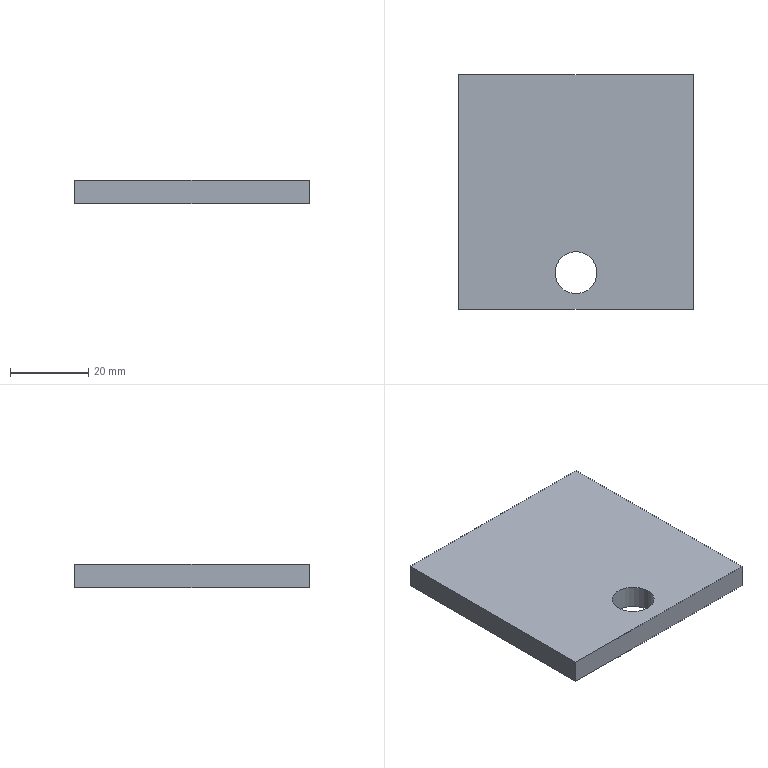Part | NX | features 凸台-拉伸21[3] 2 | 1 solid | 8 faces | box 60 x 60 x 6 mm | volume 21058 mm3 | plane 6 | cylinder 2 | commonest cylinder face diameters 10.72 x2
STEP:
#1=CARTESIAN_POINT('',(3517.64,-50.65,297.015));
#2=VERTEX_POINT('',#1);
#3=CARTESIAN_POINT('',(3517.64,-50.65,291.015));
#4=VERTEX_POINT('',#3);
#5=CARTESIAN_POINT('',(3517.64,-50.65,291.015));
#6=DIRECTION('',(0.,0.,1.));
#7=VECTOR('',#6,1000.);
#8=LINE('',#5,#7);
#9=EDGE_CURVE('',#2,#4,#8,.F.);
#10=ORIENTED_EDGE('',*,*,#9,.T.);
#11=CARTESIAN_POINT('',(3528.36,-50.65,291.015));
#12=VERTEX_POINT('',#11);
#13=CARTESIAN_POINT('',(3523.,-50.65,291.015));
#14=DIRECTION('',(0.,0.,-1.));
#15=DIRECTION('',(-1.,0.,0.));
#16=AXIS2_PLACEMENT_3D('',#13,#14,#15);
#17=CIRCLE('',#16,5.36);
#18=EDGE_CURVE('',#4,#12,#17,.T.);
#19=ORIENTED_EDGE('',*,*,#18,.T.);
#20=CARTESIAN_POINT('',(3528.36,-50.65,297.015));
#21=VERTEX_POINT('',#20);
#22=CARTESIAN_POINT('',(3528.36,-50.65,291.015));
#23=DIRECTION('',(0.,0.,1.));
#24=VECTOR('',#23,1000.);
#25=LINE('',#22,#24);
#26=EDGE_CURVE('',#12,#21,#25,.T.);
#27=ORIENTED_EDGE('',*,*,#26,.T.);
#28=CARTESIAN_POINT('',(3523.,-50.65,297.015));
#29=DIRECTION('',(0.,0.,-1.));
#30=DIRECTION('',(-1.,0.,0.));
#31=AXIS2_PLACEMENT_3D('',#28,#29,#30);
#32=CIRCLE('',#31,5.36);
#33=EDGE_CURVE('',#2,#21,#32,.T.);
#34=ORIENTED_EDGE('',*,*,#33,.F.);
#35=EDGE_LOOP('',(#10,#19,#27,#34));
#36=FACE_BOUND('',#35,.T.);
#37=CARTESIAN_POINT('',(3523.,-50.65,291.015));
#38=DIRECTION('',(0.,0.,1.));
#39=DIRECTION('',(1.,0.,0.));
#40=AXIS2_PLACEMENT_3D('',#37,#38,#39);
#41=CYLINDRICAL_SURFACE('',#40,5.36);
#42=ADVANCED_FACE('',(#36),#41,.F.);
#43=CARTESIAN_POINT('',(3493.,0.,297.015));
#44=VERTEX_POINT('',#43);
#45=CARTESIAN_POINT('',(3553.,0.,297.015));
#46=VERTEX_POINT('',#45);
#47=CARTESIAN_POINT('',(3553.,0.,297.015));
#48=DIRECTION('',(1.,0.,0.));
#49=VECTOR('',#48,1000.);
#50=LINE('',#47,#49);
#51=EDGE_CURVE('',#44,#46,#50,.T.);
#52=ORIENTED_EDGE('',*,*,#51,.T.);
#53=CARTESIAN_POINT('',(3553.,0.,291.015));
#54=VERTEX_POINT('',#53);
#55=CARTESIAN_POINT('',(3553.,0.,291.015));
#56=DIRECTION('',(0.,0.,1.));
#57=VECTOR('',#56,1000.);
#58=LINE('',#55,#57);
#59=EDGE_CURVE('',#54,#46,#58,.T.);
#60=ORIENTED_EDGE('',*,*,#59,.F.);
#61=CARTESIAN_POINT('',(3493.,0.,291.015));
#62=VERTEX_POINT('',#61);
#63=CARTESIAN_POINT('',(3553.,0.,291.015));
#64=DIRECTION('',(1.,0.,0.));
#65=VECTOR('',#64,1000.);
#66=LINE('',#63,#65);
#67=EDGE_CURVE('',#62,#54,#66,.T.);
#68=ORIENTED_EDGE('',*,*,#67,.F.);
#69=CARTESIAN_POINT('',(3493.,0.,291.015));
#70=DIRECTION('',(0.,0.,1.));
#71=VECTOR('',#70,1000.);
#72=LINE('',#69,#71);
#73=EDGE_CURVE('',#62,#44,#72,.T.);
#74=ORIENTED_EDGE('',*,*,#73,.T.);
#75=EDGE_LOOP('',(#52,#60,#68,#74));
#76=FACE_BOUND('',#75,.T.);
#77=CARTESIAN_POINT('',(3553.,0.,291.015));
#78=DIRECTION('',(0.,-1.,0.));
#79=DIRECTION('',(0.,0.,-1.));
#80=AXIS2_PLACEMENT_3D('',#77,#78,#79);
#81=PLANE('',#80);
#82=ADVANCED_FACE('',(#76),#81,.F.);
#83=CARTESIAN_POINT('',(3493.,-60.,297.015));
#84=VERTEX_POINT('',#83);
#85=CARTESIAN_POINT('',(3493.,0.,297.015));
#86=DIRECTION('',(0.,1.,0.));
#87=VECTOR('',#86,1000.);
#88=LINE('',#85,#87);
#89=EDGE_CURVE('',#84,#44,#88,.T.);
#90=ORIENTED_EDGE('',*,*,#89,.T.);
#91=ORIENTED_EDGE('',*,*,#73,.F.);
#92=CARTESIAN_POINT('',(3493.,-60.,291.015));
#93=VERTEX_POINT('',#92);
#94=CARTESIAN_POINT('',(3493.,0.,291.015));
#95=DIRECTION('',(0.,1.,0.));
#96=VECTOR('',#95,1000.);
#97=LINE('',#94,#96);
#98=EDGE_CURVE('',#93,#62,#97,.T.);
#99=ORIENTED_EDGE('',*,*,#98,.F.);
#100=CARTESIAN_POINT('',(3493.,-60.,291.015));
#101=DIRECTION('',(0.,0.,1.));
#102=VECTOR('',#101,1000.);
#103=LINE('',#100,#102);
#104=EDGE_CURVE('',#93,#84,#103,.T.);
#105=ORIENTED_EDGE('',*,*,#104,.T.);
#106=EDGE_LOOP('',(#90,#91,#99,#105));
#107=FACE_BOUND('',#106,.T.);
#108=CARTESIAN_POINT('',(3493.,0.,291.015));
#109=DIRECTION('',(1.,0.,0.));
#110=DIRECTION('',(0.,0.,-1.));
#111=AXIS2_PLACEMENT_3D('',#108,#109,#110);
#112=PLANE('',#111);
#113=ADVANCED_FACE('',(#107),#112,.F.);
#114=CARTESIAN_POINT('',(3553.,-60.,297.015));
#115=VERTEX_POINT('',#114);
#116=CARTESIAN_POINT('',(3553.,-60.,297.015));
#117=DIRECTION('',(-1.,0.,0.));
#118=VECTOR('',#117,1000.);
#119=LINE('',#116,#118);
#120=EDGE_CURVE('',#115,#84,#119,.T.);
#121=ORIENTED_EDGE('',*,*,#120,.T.);
#122=ORIENTED_EDGE('',*,*,#104,.F.);
#123=CARTESIAN_POINT('',(3553.,-60.,291.015));
#124=VERTEX_POINT('',#123);
#125=CARTESIAN_POINT('',(3553.,-60.,291.015));
#126=DIRECTION('',(-1.,0.,0.));
#127=VECTOR('',#126,1000.);
#128=LINE('',#125,#127);
#129=EDGE_CURVE('',#124,#93,#128,.T.);
#130=ORIENTED_EDGE('',*,*,#129,.F.);
#131=CARTESIAN_POINT('',(3553.,-60.,291.015));
#132=DIRECTION('',(0.,0.,1.));
#133=VECTOR('',#132,1000.);
#134=LINE('',#131,#133);
#135=EDGE_CURVE('',#124,#115,#134,.T.);
#136=ORIENTED_EDGE('',*,*,#135,.T.);
#137=EDGE_LOOP('',(#121,#122,#130,#136));
#138=FACE_BOUND('',#137,.T.);
#139=CARTESIAN_POINT('',(3553.,-60.,291.015));
#140=DIRECTION('',(0.,1.,0.));
#141=DIRECTION('',(0.,0.,1.));
#142=AXIS2_PLACEMENT_3D('',#139,#140,#141);
#143=PLANE('',#142);
#144=ADVANCED_FACE('',(#138),#143,.F.);
#145=CARTESIAN_POINT('',(3553.,0.,297.015));
#146=DIRECTION('',(0.,-1.,0.));
#147=VECTOR('',#146,1000.);
#148=LINE('',#145,#147);
#149=EDGE_CURVE('',#46,#115,#148,.T.);
#150=ORIENTED_EDGE('',*,*,#149,.T.);
#151=ORIENTED_EDGE('',*,*,#135,.F.);
#152=CARTESIAN_POINT('',(3553.,0.,291.015));
#153=DIRECTION('',(0.,-1.,0.));
#154=VECTOR('',#153,1000.);
#155=LINE('',#152,#154);
#156=EDGE_CURVE('',#54,#124,#155,.T.);
#157=ORIENTED_EDGE('',*,*,#156,.F.);
#158=ORIENTED_EDGE('',*,*,#59,.T.);
#159=EDGE_LOOP('',(#150,#151,#157,#158));
#160=FACE_BOUND('',#159,.T.);
#161=CARTESIAN_POINT('',(3553.,0.,291.015));
#162=DIRECTION('',(-1.,0.,0.));
#163=DIRECTION('',(0.,0.,1.));
#164=AXIS2_PLACEMENT_3D('',#161,#162,#163);
#165=PLANE('',#164);
#166=ADVANCED_FACE('',(#160),#165,.F.);
#167=CARTESIAN_POINT('',(3523.,-50.65,297.015));
#168=DIRECTION('',(0.,0.,-1.));
#169=DIRECTION('',(-1.,0.,0.));
#170=AXIS2_PLACEMENT_3D('',#167,#168,#169);
#171=CIRCLE('',#170,5.36);
#172=EDGE_CURVE('',#21,#2,#171,.T.);
#173=ORIENTED_EDGE('',*,*,#172,.T.);
#174=ORIENTED_EDGE('',*,*,#33,.T.);
#175=EDGE_LOOP('',(#173,#174));
#176=FACE_BOUND('',#175,.T.);
#177=ORIENTED_EDGE('',*,*,#149,.F.);
#178=ORIENTED_EDGE('',*,*,#51,.F.);
#179=ORIENTED_EDGE('',*,*,#89,.F.);
#180=ORIENTED_EDGE('',*,*,#120,.F.);
#181=EDGE_LOOP('',(#177,#178,#179,#180));
#182=FACE_BOUND('',#181,.T.);
#183=CARTESIAN_POINT('',(3000.,0.,297.015));
#184=DIRECTION('',(0.,0.,-1.));
#185=DIRECTION('',(-1.,0.,0.));
#186=AXIS2_PLACEMENT_3D('',#183,#184,#185);
#187=PLANE('',#186);
#188=ADVANCED_FACE('',(#176,#182),#187,.F.);
#189=CARTESIAN_POINT('',(3523.,-50.65,291.015));
#190=DIRECTION('',(0.,0.,-1.));
#191=DIRECTION('',(-1.,0.,0.));
#192=AXIS2_PLACEMENT_3D('',#189,#190,#191);
#193=CIRCLE('',#192,5.36);
#194=EDGE_CURVE('',#12,#4,#193,.T.);
#195=ORIENTED_EDGE('',*,*,#194,.F.);
#196=ORIENTED_EDGE('',*,*,#18,.F.);
#197=EDGE_LOOP('',(#195,#196));
#198=FACE_BOUND('',#197,.T.);
#199=ORIENTED_EDGE('',*,*,#156,.T.);
#200=ORIENTED_EDGE('',*,*,#129,.T.);
#201=ORIENTED_EDGE('',*,*,#98,.T.);
#202=ORIENTED_EDGE('',*,*,#67,.T.);
#203=EDGE_LOOP('',(#199,#200,#201,#202));
#204=FACE_BOUND('',#203,.T.);
#205=CARTESIAN_POINT('',(3000.,0.,291.015));
#206=DIRECTION('',(0.,0.,-1.));
#207=DIRECTION('',(-1.,0.,0.));
#208=AXIS2_PLACEMENT_3D('',#205,#206,#207);
#209=PLANE('',#208);
#210=ADVANCED_FACE('',(#198,#204),#209,.T.);
#211=ORIENTED_EDGE('',*,*,#194,.T.);
#212=ORIENTED_EDGE('',*,*,#9,.F.);
#213=ORIENTED_EDGE('',*,*,#172,.F.);
#214=ORIENTED_EDGE('',*,*,#26,.F.);
#215=EDGE_LOOP('',(#211,#212,#213,#214));
#216=FACE_BOUND('',#215,.T.);
#217=CARTESIAN_POINT('',(3523.,-50.65,291.015));
#218=DIRECTION('',(0.,0.,1.));
#219=DIRECTION('',(1.,0.,0.));
#220=AXIS2_PLACEMENT_3D('',#217,#218,#219);
#221=CYLINDRICAL_SURFACE('',#220,5.36);
#222=ADVANCED_FACE('',(#216),#221,.F.);
#223=CLOSED_SHELL('',(#42,#82,#113,#144,#166,#188,#210,#222));
#224=MANIFOLD_SOLID_BREP('',#223);
#225=(LENGTH_UNIT()NAMED_UNIT(*)SI_UNIT(.MILLI.,.METRE.));
#226=UNCERTAINTY_MEASURE_WITH_UNIT(LENGTH_MEASURE(0.00001),#225,'','');
#227=(NAMED_UNIT(*)PLANE_ANGLE_UNIT()SI_UNIT($,.RADIAN.));
#228=(NAMED_UNIT(*)SI_UNIT($,.STERADIAN.)SOLID_ANGLE_UNIT());
#229=(GEOMETRIC_REPRESENTATION_CONTEXT(3)GLOBAL_UNCERTAINTY_ASSIGNED_CONTEXT((#226))GLOBAL_UNIT_ASSIGNED_CONTEXT((#225,#227,#228))REPRESENTATION_CONTEXT('',''));
#230=ADVANCED_BREP_SHAPE_REPRESENTATION('',(#224),#229);